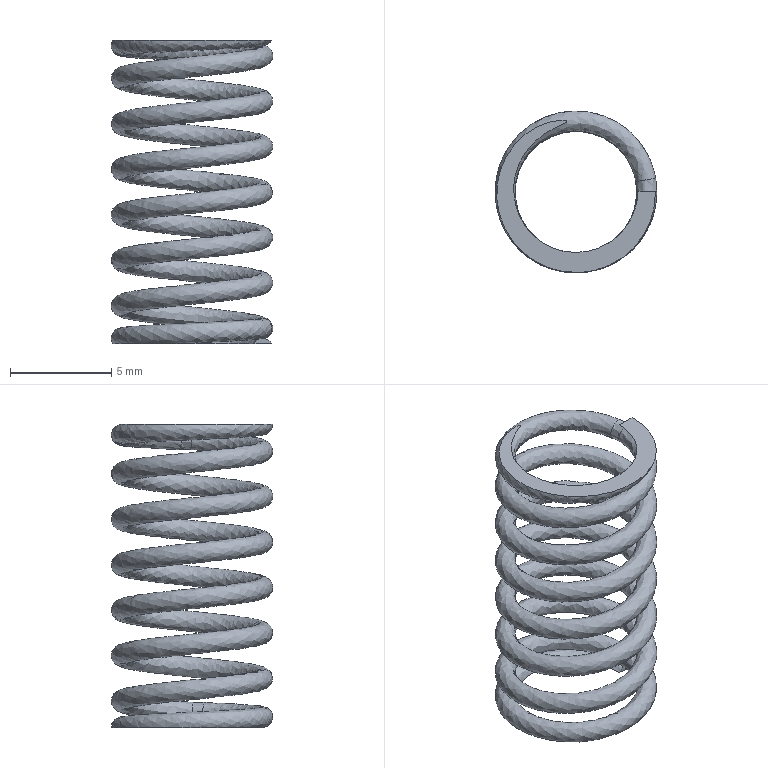Part | STEP file | 1 solid | 9 faces | volume 125.363 mm3 | spline 5 | plane 4